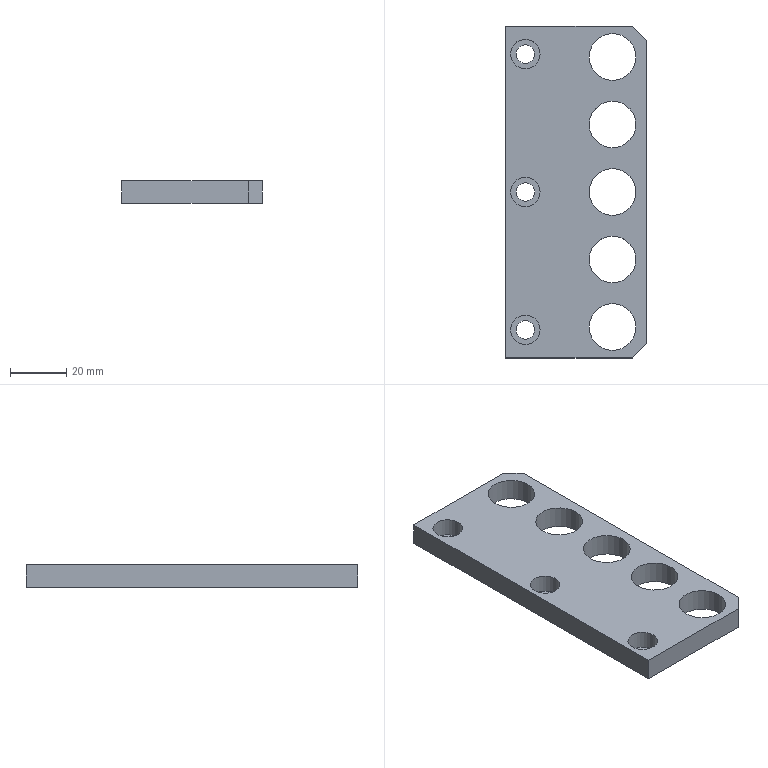NC program | NX | posted with a generic post | part box 50 x 118 x 8 mm
Lines 2317 to 2555 of 2555:
(PLANAR_MILL_2 , TOOL : D4点钻)
N4608 T05 M6
N4610 G54
N4612 G17 G0 G90 X61.828 Y-26. S3000 M3
N4614 G43 Z30. H5
N4616 Z1.
N4618 G94 G1 Z-1. F800.
N4620 X58.999
N4622 X-59.
N4624 G2 X-60. Y-25. R1.
N4626 G1 Y20.
N4628 G2 X-59.707 Y20.707 R1.
N4630 G1 X-54.707 Y25.707
N4632 G2 X-54. Y26. R1.
N4634 G1 X54.
N4636 G2 X54.707 Y25.707 R1.
N4638 G1 X59.707 Y20.707
N4640 G2 X60. Y20. R1.
N4642 G1 Y-24.999
N4644 Y-27.828
N4646 Z1.
N4648 G0 Z30.
(PLANAR_MILL_2_COPY , TOOL : D4点钻)
N4650 X-50. Y8.092
N4652 Z1.
N4654 G1 Z-1.
N4656 Y7.7
N4658 G3 X-48. Y5.7 R2.
N4660 X-40.7 Y13. R7.3
N4662 X-48. Y5.7 R-7.3
N4664 X-46. Y7.7 R2.
N4666 G1 Y8.092
N4668 Z1.
N4670 G0 Z30.
N4672 X-26.
N4674 Z1.
N4676 G1 Z-1.
N4678 Y7.7
N4680 G3 X-24. Y5.7 R2.
N4682 X-16.7 Y13. R7.3
N4684 X-24. Y5.7 R-7.3
N4686 X-22. Y7.7 R2.
N4688 G1 Y8.092
N4690 Z1.
N4692 G0 Z30.
N4694 X-2.
N4696 Z1.
N4698 G1 Z-1.
N4700 Y7.7
N4702 G3 X0. Y5.7 R2.
N4704 X7.3 Y13. R7.3
N4706 X0. Y5.7 R-7.3
N4708 X2. Y7.7 R2.
N4710 G1 Y8.092
N4712 Z1.
N4714 G0 Z30.
N4716 X22.
N4718 Z1.
N4720 G1 Z-1.
N4722 Y7.7
N4724 G3 X24. Y5.7 R2.
N4726 X31.3 Y13. R7.3
N4728 X24. Y5.7 R-7.3
N4730 X26. Y7.7 R2.
N4732 G1 Y8.092
N4734 Z1.
N4736 G0 Z30.
N4738 X46.
N4740 Z1.
N4742 G1 Z-1.
N4744 Y7.7
N4746 G3 X48. Y5.7 R2.
N4748 X55.3 Y13. R7.3
N4750 X48. Y5.7 R-7.3
N4752 X50. Y7.7 R2.
N4754 G1 Y8.092
N4756 Z1.
N4758 G0 Z30.
(PLANAR_MILL_2_COPY_COPY , TOOL : D4点钻)
N4760 X-48. Y-14.908
N4762 Z1.
N4764 G1 Z-1.
N4766 Y-14.75
N4768 G3 X-49. Y-13.75 R1.
N4770 X-53.25 Y-18. R4.25
N4772 X-49. Y-13.75 R-4.25
N4774 X-50. Y-14.75 R1.
N4776 G1 Y-14.908
N4778 Z1.
N4780 G0 Z30.
N4782 X-1. Y-21.092
N4784 Z1.
N4786 G1 Z-1.
N4788 Y-21.25
N4790 G3 X0. Y-22.25 R1.
N4792 X4.25 Y-18. R4.25
N4794 X0. Y-22.25 R-4.25
N4796 X1. Y-21.25 R1.
N4798 G1 Y-21.092
N4800 Z1.
N4802 G0 Z30.
N4804 X48.
N4806 Z1.
N4808 G1 Z-1.
N4810 Y-21.25
N4812 G3 X49. Y-22.25 R1.
N4814 X53.25 Y-18. R4.25
N4816 X49. Y-22.25 R-4.25
N4818 X50. Y-21.25 R1.
N4820 G1 Y-21.092
N4822 Z1.
N4824 G0 Z30.
N4826 M5
(PLANAR_MILL_3 , TOOL : D6精光)
N4828 T06 M6
N4830 G54
N4832 G17 G0 G90 X63. Y-28. S3500 M3
N4834 G43 Z30. H6
N4836 Z-7.
N4838 G94 G1 Z-9. F800.
N4840 X58.999
N4842 X-59.
N4844 G2 X-62. Y-25. R3.
N4846 G1 Y20.
N4848 G2 X-61.121 Y22.121 R3.
N4850 G1 X-56.121 Y27.121
N4852 G2 X-54. Y28. R3.
N4854 G1 X54.
N4856 G2 X56.121 Y27.121 R3.
N4858 G1 X61.121 Y22.121
N4860 G2 X62. Y20. R3.
N4862 G1 Y-24.999
N4864 Y-29.
N4866 Z-7.
N4868 G0 Z30.
(PLANAR_MILL_4 , TOOL : D6精光)
N4870 X50. Y15.625
N4872 Z-7.
N4874 G1 Z-9.
N4876 Y16.3
N4878 G3 X48. Y18.3 R2.
N4880 X42.7 Y13. R5.3
N4882 X48. Y18.3 R-5.3
N4884 X46. Y16.3 R2.
N4886 G1 Y15.625
N4888 Z-7.
N4890 G0 Z30.
N4892 X26.
N4894 Z-7.
N4896 G1 Z-9.
N4898 Y16.3
N4900 G3 X24. Y18.3 R2.
N4902 X18.7 Y13. R5.3
N4904 X24. Y18.3 R-5.3
N4906 X22. Y16.3 R2.
N4908 G1 Y15.625
N4910 Z-7.
N4912 G0 Z30.
N4914 X2.
N4916 Z-7.
N4918 G1 Z-9.
N4920 Y16.3
N4922 G3 X0. Y18.3 R2.
N4924 X-5.3 Y13. R5.3
N4926 X0. Y18.3 R-5.3
N4928 X-2. Y16.3 R2.
N4930 G1 Y15.625
N4932 Z-7.
N4934 G0 Z30.
N4936 X-22.
N4938 Z-7.
N4940 G1 Z-9.
N4942 Y16.3
N4944 G3 X-24. Y18.3 R2.
N4946 X-29.3 Y13. R5.3
N4948 X-24. Y18.3 R-5.3
N4950 X-26. Y16.3 R2.
N4952 G1 Y15.625
N4954 Z-7.
N4956 G0 Z30.
N4958 X-46.
N4960 Z-7.
N4962 G1 Z-9.
N4964 Y16.3
N4966 G3 X-48. Y18.3 R2.
N4968 X-53.3 Y13. R5.3
N4970 X-48. Y18.3 R-5.3
N4972 X-50. Y16.3 R2.
N4974 G1 Y15.625
N4976 Z-7.
N4978 G0 Z30.
(PLANAR_MILL_5 , TOOL : D6精光)
N4980 X-49. Y-18.25
N4982 Z-4.5
N4984 G1 Z-6.5
N4986 X-51.
N4988 G3 X-49. Y-20.25 R2.
N4990 X-46.75 Y-18. R2.25
N4992 X-49. Y-20.25 R-2.25
N4994 X-47. Y-18.25 R2.
N4996 G1 X-49.
N4998 Z-4.5
N5000 G0 Z30.
N5002 X0. Y-17.75
N5004 Z-4.5
N5006 G1 Z-6.5
N5008 X2.
N5010 G3 X0. Y-15.75 R2.
N5012 X-2.25 Y-18. R2.25
N5014 X0. Y-15.75 R-2.25
N5016 X-2. Y-17.75 R2.
N5018 G1 X0.
N5020 Z-4.5
N5022 G0 Z30.
N5024 X49.
N5026 Z-4.5
N5028 G1 Z-6.5
N5030 X51.
N5032 G3 X49. Y-15.75 R2.
N5034 X46.75 Y-18. R2.25
N5036 X49. Y-15.75 R-2.25
N5038 X47. Y-17.75 R2.
N5040 G1 X49.
N5042 Z-4.5
N5044 G0 Z30.
N5046 M5
N5048 M2